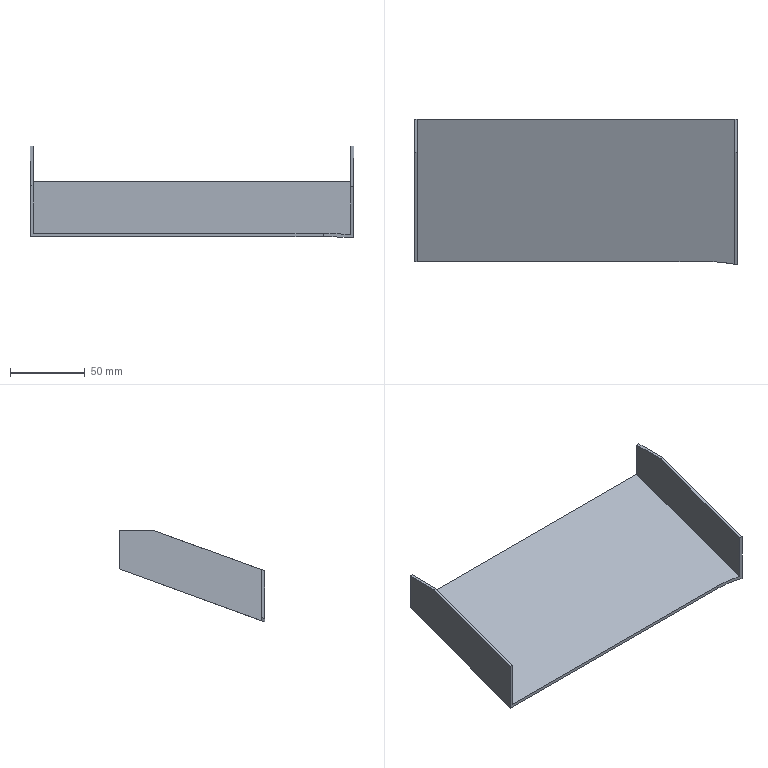Part | NX | features HB 2 | 1 solid | 13 faces | box 216 x 97.247 x 61.333 mm | volume 55606 mm3 | plane 12 | cylinder 1 | commonest cylinder face diameters 190 x1
STEP:
#1=CARTESIAN_POINT('',(865.54,217.702,-213.));
#2=VERTEX_POINT('',#1);
#3=CARTESIAN_POINT('',(865.54,240.,-213.));
#4=VERTEX_POINT('',#3);
#5=CARTESIAN_POINT('',(865.54,20.77,-213.));
#6=DIRECTION('',(0.,1.,0.));
#7=VECTOR('',#6,1000.);
#8=LINE('',#5,#7);
#9=EDGE_CURVE('',#2,#4,#8,.T.);
#10=ORIENTED_EDGE('',*,*,#9,.F.);
#11=CARTESIAN_POINT('',(865.54,142.753,-240.279));
#12=VERTEX_POINT('',#11);
#13=CARTESIAN_POINT('',(865.54,10.51,-288.412));
#14=DIRECTION('',(0.,0.9397,0.342));
#15=VECTOR('',#14,1000.);
#16=LINE('',#13,#15);
#17=EDGE_CURVE('',#12,#2,#16,.T.);
#18=ORIENTED_EDGE('',*,*,#17,.F.);
#19=CARTESIAN_POINT('',(865.54,142.753,-274.333));
#20=VERTEX_POINT('',#19);
#21=CARTESIAN_POINT('',(865.54,142.753,-1420.5));
#22=DIRECTION('',(0.,0.,1.));
#23=VECTOR('',#22,1000.);
#24=LINE('',#21,#23);
#25=EDGE_CURVE('',#20,#12,#24,.T.);
#26=ORIENTED_EDGE('',*,*,#25,.F.);
#27=CARTESIAN_POINT('',(865.54,240.,-238.938));
#28=VERTEX_POINT('',#27);
#29=CARTESIAN_POINT('',(865.54,21.454,-318.482));
#30=DIRECTION('',(0.,-0.9397,-0.342));
#31=VECTOR('',#30,1000.);
#32=LINE('',#29,#31);
#33=EDGE_CURVE('',#28,#20,#32,.T.);
#34=ORIENTED_EDGE('',*,*,#33,.F.);
#35=CARTESIAN_POINT('',(865.54,240.,-316.603));
#36=DIRECTION('',(0.,0.,-1.));
#37=VECTOR('',#36,1000.);
#38=LINE('',#35,#37);
#39=EDGE_CURVE('',#4,#28,#38,.T.);
#40=ORIENTED_EDGE('',*,*,#39,.F.);
#41=EDGE_LOOP('',(#10,#18,#26,#34,#40));
#42=FACE_BOUND('',#41,.T.);
#43=CARTESIAN_POINT('',(865.54,20.77,-316.603));
#44=DIRECTION('',(-1.,0.,0.));
#45=DIRECTION('',(0.,-0.08716,-0.9962));
#46=AXIS2_PLACEMENT_3D('',#43,#44,#45);
#47=PLANE('',#46);
#48=ADVANCED_FACE('',(#42),#47,.F.);
#49=CARTESIAN_POINT('',(649.54,240.,-213.));
#50=VERTEX_POINT('',#49);
#51=CARTESIAN_POINT('',(649.54,217.702,-213.));
#52=VERTEX_POINT('',#51);
#53=CARTESIAN_POINT('',(649.54,20.77,-213.));
#54=DIRECTION('',(0.,-1.,0.));
#55=VECTOR('',#54,1000.);
#56=LINE('',#53,#55);
#57=EDGE_CURVE('',#50,#52,#56,.T.);
#58=ORIENTED_EDGE('',*,*,#57,.F.);
#59=CARTESIAN_POINT('',(649.54,240.,-238.938));
#60=VERTEX_POINT('',#59);
#61=CARTESIAN_POINT('',(649.54,240.,-316.603));
#62=DIRECTION('',(0.,0.,1.));
#63=VECTOR('',#62,1000.);
#64=LINE('',#61,#63);
#65=EDGE_CURVE('',#60,#50,#64,.T.);
#66=ORIENTED_EDGE('',*,*,#65,.F.);
#67=CARTESIAN_POINT('',(649.54,145.,-273.515));
#68=VERTEX_POINT('',#67);
#69=CARTESIAN_POINT('',(649.54,21.454,-318.482));
#70=DIRECTION('',(0.,0.9397,0.342));
#71=VECTOR('',#70,1000.);
#72=LINE('',#69,#71);
#73=EDGE_CURVE('',#68,#60,#72,.T.);
#74=ORIENTED_EDGE('',*,*,#73,.F.);
#75=CARTESIAN_POINT('',(649.54,145.,-239.462));
#76=VERTEX_POINT('',#75);
#77=CARTESIAN_POINT('',(649.54,145.,-316.603));
#78=DIRECTION('',(0.,0.,-1.));
#79=VECTOR('',#78,1000.);
#80=LINE('',#77,#79);
#81=EDGE_CURVE('',#76,#68,#80,.T.);
#82=ORIENTED_EDGE('',*,*,#81,.F.);
#83=CARTESIAN_POINT('',(649.54,10.51,-288.412));
#84=DIRECTION('',(0.,0.9397,0.342));
#85=VECTOR('',#84,1000.);
#86=LINE('',#83,#85);
#87=EDGE_CURVE('',#76,#52,#86,.T.);
#88=ORIENTED_EDGE('',*,*,#87,.T.);
#89=EDGE_LOOP('',(#58,#66,#74,#82,#88));
#90=FACE_BOUND('',#89,.T.);
#91=CARTESIAN_POINT('',(649.54,20.77,-316.603));
#92=DIRECTION('',(1.,0.,0.));
#93=DIRECTION('',(0.,0.08716,0.9962));
#94=AXIS2_PLACEMENT_3D('',#91,#92,#93);
#95=PLANE('',#94);
#96=ADVANCED_FACE('',(#90),#95,.F.);
#97=CARTESIAN_POINT('',(651.54,240.,-236.81));
#98=VERTEX_POINT('',#97);
#99=CARTESIAN_POINT('',(651.54,240.,-213.));
#100=VERTEX_POINT('',#99);
#101=CARTESIAN_POINT('',(651.54,240.,-316.603));
#102=DIRECTION('',(0.,0.,1.));
#103=VECTOR('',#102,1000.);
#104=LINE('',#101,#103);
#105=EDGE_CURVE('',#98,#100,#104,.T.);
#106=ORIENTED_EDGE('',*,*,#105,.T.);
#107=CARTESIAN_POINT('',(651.54,217.702,-213.));
#108=VERTEX_POINT('',#107);
#109=CARTESIAN_POINT('',(651.54,20.77,-213.));
#110=DIRECTION('',(0.,-1.,0.));
#111=VECTOR('',#110,1000.);
#112=LINE('',#109,#111);
#113=EDGE_CURVE('',#100,#108,#112,.T.);
#114=ORIENTED_EDGE('',*,*,#113,.T.);
#115=CARTESIAN_POINT('',(651.54,145.,-239.462));
#116=VERTEX_POINT('',#115);
#117=CARTESIAN_POINT('',(651.54,10.51,-288.412));
#118=DIRECTION('',(0.,0.9397,0.342));
#119=VECTOR('',#118,1000.);
#120=LINE('',#117,#119);
#121=EDGE_CURVE('',#116,#108,#120,.T.);
#122=ORIENTED_EDGE('',*,*,#121,.F.);
#123=CARTESIAN_POINT('',(651.54,145.,-271.387));
#124=VERTEX_POINT('',#123);
#125=CARTESIAN_POINT('',(651.54,145.,-1420.5));
#126=DIRECTION('',(0.,0.,1.));
#127=VECTOR('',#126,1000.);
#128=LINE('',#125,#127);
#129=EDGE_CURVE('',#124,#116,#128,.T.);
#130=ORIENTED_EDGE('',*,*,#129,.F.);
#131=CARTESIAN_POINT('',(651.54,20.77,-316.603));
#132=DIRECTION('',(0.,-0.9397,-0.342));
#133=VECTOR('',#132,1000.);
#134=LINE('',#131,#133);
#135=EDGE_CURVE('',#98,#124,#134,.T.);
#136=ORIENTED_EDGE('',*,*,#135,.F.);
#137=EDGE_LOOP('',(#106,#114,#122,#130,#136));
#138=FACE_BOUND('',#137,.T.);
#139=CARTESIAN_POINT('',(651.54,20.77,-316.603));
#140=DIRECTION('',(1.,0.,0.));
#141=DIRECTION('',(0.,0.08716,0.9962));
#142=AXIS2_PLACEMENT_3D('',#139,#140,#141);
#143=PLANE('',#142);
#144=ADVANCED_FACE('',(#138),#143,.T.);
#145=CARTESIAN_POINT('',(863.54,143.173,-240.126));
#146=VERTEX_POINT('',#145);
#147=CARTESIAN_POINT('',(863.54,217.702,-213.));
#148=VERTEX_POINT('',#147);
#149=CARTESIAN_POINT('',(863.54,10.51,-288.412));
#150=DIRECTION('',(0.,0.9397,0.342));
#151=VECTOR('',#150,1000.);
#152=LINE('',#149,#151);
#153=EDGE_CURVE('',#146,#148,#152,.T.);
#154=ORIENTED_EDGE('',*,*,#153,.T.);
#155=CARTESIAN_POINT('',(863.54,240.,-213.));
#156=VERTEX_POINT('',#155);
#157=CARTESIAN_POINT('',(863.54,20.77,-213.));
#158=DIRECTION('',(0.,1.,0.));
#159=VECTOR('',#158,1000.);
#160=LINE('',#157,#159);
#161=EDGE_CURVE('',#148,#156,#160,.T.);
#162=ORIENTED_EDGE('',*,*,#161,.T.);
#163=CARTESIAN_POINT('',(863.54,240.,-236.81));
#164=VERTEX_POINT('',#163);
#165=CARTESIAN_POINT('',(863.54,240.,-316.603));
#166=DIRECTION('',(0.,0.,-1.));
#167=VECTOR('',#166,1000.);
#168=LINE('',#165,#167);
#169=EDGE_CURVE('',#156,#164,#168,.T.);
#170=ORIENTED_EDGE('',*,*,#169,.T.);
#171=CARTESIAN_POINT('',(863.54,143.173,-272.052));
#172=VERTEX_POINT('',#171);
#173=CARTESIAN_POINT('',(863.54,20.77,-316.603));
#174=DIRECTION('',(0.,0.9397,0.342));
#175=VECTOR('',#174,1000.);
#176=LINE('',#173,#175);
#177=EDGE_CURVE('',#172,#164,#176,.T.);
#178=ORIENTED_EDGE('',*,*,#177,.F.);
#179=CARTESIAN_POINT('',(863.54,143.173,-1420.5));
#180=DIRECTION('',(0.,0.,1.));
#181=VECTOR('',#180,1000.);
#182=LINE('',#179,#181);
#183=EDGE_CURVE('',#172,#146,#182,.T.);
#184=ORIENTED_EDGE('',*,*,#183,.T.);
#185=EDGE_LOOP('',(#154,#162,#170,#178,#184));
#186=FACE_BOUND('',#185,.T.);
#187=CARTESIAN_POINT('',(863.54,20.77,-316.603));
#188=DIRECTION('',(-1.,0.,0.));
#189=DIRECTION('',(0.,0.08716,0.9962));
#190=AXIS2_PLACEMENT_3D('',#187,#188,#189);
#191=PLANE('',#190);
#192=ADVANCED_FACE('',(#186),#191,.T.);
#193=CARTESIAN_POINT('',(651.54,217.702,-213.));
#194=DIRECTION('',(1.,0.,0.));
#195=VECTOR('',#194,1000.);
#196=LINE('',#193,#195);
#197=EDGE_CURVE('',#52,#108,#196,.T.);
#198=ORIENTED_EDGE('',*,*,#197,.F.);
#199=ORIENTED_EDGE('',*,*,#87,.F.);
#200=CARTESIAN_POINT('',(651.54,145.,-239.462));
#201=DIRECTION('',(-1.,0.,0.));
#202=VECTOR('',#201,1000.);
#203=LINE('',#200,#202);
#204=EDGE_CURVE('',#116,#76,#203,.T.);
#205=ORIENTED_EDGE('',*,*,#204,.F.);
#206=ORIENTED_EDGE('',*,*,#121,.T.);
#207=EDGE_LOOP('',(#198,#199,#205,#206));
#208=FACE_BOUND('',#207,.T.);
#209=CARTESIAN_POINT('',(651.54,10.51,-288.412));
#210=DIRECTION('',(0.,0.342,-0.9397));
#211=DIRECTION('',(0.,-0.9397,-0.342));
#212=AXIS2_PLACEMENT_3D('',#209,#210,#211);
#213=PLANE('',#212);
#214=ADVANCED_FACE('',(#208),#213,.F.);
#215=CARTESIAN_POINT('',(973.54,217.702,-213.));
#216=DIRECTION('',(1.,0.,0.));
#217=VECTOR('',#216,1000.);
#218=LINE('',#215,#217);
#219=EDGE_CURVE('',#148,#2,#218,.T.);
#220=ORIENTED_EDGE('',*,*,#219,.F.);
#221=ORIENTED_EDGE('',*,*,#153,.F.);
#222=CARTESIAN_POINT('',(845.,50.,-274.039));
#223=DIRECTION('',(0.,-0.342,0.9397));
#224=DIRECTION('',(0.,0.9397,0.342));
#225=AXIS2_PLACEMENT_3D('',#222,#223,#224);
#226=ELLIPSE('',#225,101.097,95.);
#227=EDGE_CURVE('',#12,#146,#226,.T.);
#228=ORIENTED_EDGE('',*,*,#227,.F.);
#229=ORIENTED_EDGE('',*,*,#17,.T.);
#230=EDGE_LOOP('',(#220,#221,#228,#229));
#231=FACE_BOUND('',#230,.T.);
#232=CARTESIAN_POINT('',(973.54,10.51,-288.412));
#233=DIRECTION('',(0.,0.342,-0.9397));
#234=DIRECTION('',(0.,-0.9397,-0.342));
#235=AXIS2_PLACEMENT_3D('',#232,#233,#234);
#236=PLANE('',#235);
#237=ADVANCED_FACE('',(#231),#236,.F.);
#238=ORIENTED_EDGE('',*,*,#65,.T.);
#239=CARTESIAN_POINT('',(977.,240.,-213.));
#240=DIRECTION('',(1.,0.,0.));
#241=VECTOR('',#240,1000.);
#242=LINE('',#239,#241);
#243=EDGE_CURVE('',#50,#100,#242,.T.);
#244=ORIENTED_EDGE('',*,*,#243,.T.);
#245=ORIENTED_EDGE('',*,*,#105,.F.);
#246=CARTESIAN_POINT('',(868.54,240.,-236.81));
#247=DIRECTION('',(-1.,0.,0.));
#248=VECTOR('',#247,1000.);
#249=LINE('',#246,#248);
#250=EDGE_CURVE('',#164,#98,#249,.T.);
#251=ORIENTED_EDGE('',*,*,#250,.F.);
#252=ORIENTED_EDGE('',*,*,#169,.F.);
#253=CARTESIAN_POINT('',(962.,240.,-213.));
#254=DIRECTION('',(1.,0.,0.));
#255=VECTOR('',#254,1000.);
#256=LINE('',#253,#255);
#257=EDGE_CURVE('',#156,#4,#256,.T.);
#258=ORIENTED_EDGE('',*,*,#257,.T.);
#259=ORIENTED_EDGE('',*,*,#39,.T.);
#260=CARTESIAN_POINT('',(868.54,240.,-238.938));
#261=DIRECTION('',(-1.,0.,0.));
#262=VECTOR('',#261,1000.);
#263=LINE('',#260,#262);
#264=EDGE_CURVE('',#28,#60,#263,.T.);
#265=ORIENTED_EDGE('',*,*,#264,.T.);
#266=EDGE_LOOP('',(#238,#244,#245,#251,#252,#258,#259,#265));
#267=FACE_BOUND('',#266,.T.);
#268=CARTESIAN_POINT('',(962.,240.,60.));
#269=DIRECTION('',(0.,1.,0.));
#270=DIRECTION('',(0.,0.,-1.));
#271=AXIS2_PLACEMENT_3D('',#268,#269,#270);
#272=PLANE('',#271);
#273=ADVANCED_FACE('',(#267),#272,.T.);
#274=ORIENTED_EDGE('',*,*,#135,.T.);
#275=CARTESIAN_POINT('',(845.,145.,-271.387));
#276=VERTEX_POINT('',#275);
#277=CARTESIAN_POINT('',(868.54,145.,-271.387));
#278=DIRECTION('',(1.,0.,0.));
#279=VECTOR('',#278,1000.);
#280=LINE('',#277,#279);
#281=EDGE_CURVE('',#124,#276,#280,.T.);
#282=ORIENTED_EDGE('',*,*,#281,.T.);
#283=CARTESIAN_POINT('',(845.,50.,-305.964));
#284=DIRECTION('',(0.,-0.342,0.9397));
#285=DIRECTION('',(0.,0.9397,0.342));
#286=AXIS2_PLACEMENT_3D('',#283,#284,#285);
#287=ELLIPSE('',#286,101.097,95.);
#288=EDGE_CURVE('',#172,#276,#287,.T.);
#289=ORIENTED_EDGE('',*,*,#288,.F.);
#290=ORIENTED_EDGE('',*,*,#177,.T.);
#291=ORIENTED_EDGE('',*,*,#250,.T.);
#292=EDGE_LOOP('',(#274,#282,#289,#290,#291));
#293=FACE_BOUND('',#292,.T.);
#294=CARTESIAN_POINT('',(868.54,20.77,-316.603));
#295=DIRECTION('',(0.,-0.342,0.9397));
#296=DIRECTION('',(-1.,0.,0.));
#297=AXIS2_PLACEMENT_3D('',#294,#295,#296);
#298=PLANE('',#297);
#299=ADVANCED_FACE('',(#293),#298,.T.);
#300=CARTESIAN_POINT('',(845.,145.,-273.515));
#301=VERTEX_POINT('',#300);
#302=CARTESIAN_POINT('',(868.54,145.,-273.515));
#303=DIRECTION('',(-1.,0.,0.));
#304=VECTOR('',#303,1000.);
#305=LINE('',#302,#304);
#306=EDGE_CURVE('',#301,#68,#305,.T.);
#307=ORIENTED_EDGE('',*,*,#306,.T.);
#308=ORIENTED_EDGE('',*,*,#73,.T.);
#309=ORIENTED_EDGE('',*,*,#264,.F.);
#310=ORIENTED_EDGE('',*,*,#33,.T.);
#311=CARTESIAN_POINT('',(845.,50.,-308.092));
#312=DIRECTION('',(0.,-0.342,0.9397));
#313=DIRECTION('',(0.,0.9397,0.342));
#314=AXIS2_PLACEMENT_3D('',#311,#312,#313);
#315=ELLIPSE('',#314,101.097,95.);
#316=EDGE_CURVE('',#20,#301,#315,.T.);
#317=ORIENTED_EDGE('',*,*,#316,.T.);
#318=EDGE_LOOP('',(#307,#308,#309,#310,#317));
#319=FACE_BOUND('',#318,.T.);
#320=CARTESIAN_POINT('',(868.54,21.454,-318.482));
#321=DIRECTION('',(0.,-0.342,0.9397));
#322=DIRECTION('',(-1.,0.,0.));
#323=AXIS2_PLACEMENT_3D('',#320,#321,#322);
#324=PLANE('',#323);
#325=ADVANCED_FACE('',(#319),#324,.F.);
#326=ORIENTED_EDGE('',*,*,#281,.F.);
#327=ORIENTED_EDGE('',*,*,#129,.T.);
#328=ORIENTED_EDGE('',*,*,#204,.T.);
#329=ORIENTED_EDGE('',*,*,#81,.T.);
#330=ORIENTED_EDGE('',*,*,#306,.F.);
#331=CARTESIAN_POINT('',(845.,145.,-1420.5));
#332=DIRECTION('',(0.,0.,1.));
#333=VECTOR('',#332,1000.);
#334=LINE('',#331,#333);
#335=EDGE_CURVE('',#301,#276,#334,.T.);
#336=ORIENTED_EDGE('',*,*,#335,.T.);
#337=EDGE_LOOP('',(#326,#327,#328,#329,#330,#336));
#338=FACE_BOUND('',#337,.T.);
#339=CARTESIAN_POINT('',(645.,145.,-1420.5));
#340=DIRECTION('',(0.,-1.,0.));
#341=DIRECTION('',(0.,0.,1.));
#342=AXIS2_PLACEMENT_3D('',#339,#340,#341);
#343=PLANE('',#342);
#344=ADVANCED_FACE('',(#338),#343,.T.);
#345=ORIENTED_EDGE('',*,*,#288,.T.);
#346=ORIENTED_EDGE('',*,*,#335,.F.);
#347=ORIENTED_EDGE('',*,*,#316,.F.);
#348=ORIENTED_EDGE('',*,*,#25,.T.);
#349=ORIENTED_EDGE('',*,*,#227,.T.);
#350=ORIENTED_EDGE('',*,*,#183,.F.);
#351=EDGE_LOOP('',(#345,#346,#347,#348,#349,#350));
#352=FACE_BOUND('',#351,.T.);
#353=CARTESIAN_POINT('',(845.,50.,-1420.5));
#354=DIRECTION('',(0.,0.,1.));
#355=DIRECTION('',(-1.,0.,0.));
#356=AXIS2_PLACEMENT_3D('',#353,#354,#355);
#357=CYLINDRICAL_SURFACE('',#356,95.);
#358=ADVANCED_FACE('',(#352),#357,.F.);
#359=ORIENTED_EDGE('',*,*,#161,.F.);
#360=ORIENTED_EDGE('',*,*,#219,.T.);
#361=ORIENTED_EDGE('',*,*,#9,.T.);
#362=ORIENTED_EDGE('',*,*,#257,.F.);
#363=EDGE_LOOP('',(#359,#360,#361,#362));
#364=FACE_BOUND('',#363,.T.);
#365=CARTESIAN_POINT('',(1945.,0.,-213.));
#366=DIRECTION('',(0.,0.,1.));
#367=DIRECTION('',(-1.,0.,0.));
#368=AXIS2_PLACEMENT_3D('',#365,#366,#367);
#369=PLANE('',#368);
#370=ADVANCED_FACE('',(#364),#369,.T.);
#371=ORIENTED_EDGE('',*,*,#57,.T.);
#372=ORIENTED_EDGE('',*,*,#197,.T.);
#373=ORIENTED_EDGE('',*,*,#113,.F.);
#374=ORIENTED_EDGE('',*,*,#243,.F.);
#375=EDGE_LOOP('',(#371,#372,#373,#374));
#376=FACE_BOUND('',#375,.T.);
#377=CARTESIAN_POINT('',(1960.,0.,-213.));
#378=DIRECTION('',(0.,0.,1.));
#379=DIRECTION('',(-1.,0.,0.));
#380=AXIS2_PLACEMENT_3D('',#377,#378,#379);
#381=PLANE('',#380);
#382=ADVANCED_FACE('',(#376),#381,.T.);
#383=CLOSED_SHELL('',(#48,#96,#144,#192,#214,#237,#273,#299,#325,#344,#358,#370,#382));
#384=MANIFOLD_SOLID_BREP('',#383);
#385=(LENGTH_UNIT()NAMED_UNIT(*)SI_UNIT(.MILLI.,.METRE.));
#386=UNCERTAINTY_MEASURE_WITH_UNIT(LENGTH_MEASURE(0.00001),#385,'','');
#387=(NAMED_UNIT(*)PLANE_ANGLE_UNIT()SI_UNIT($,.RADIAN.));
#388=(NAMED_UNIT(*)SI_UNIT($,.STERADIAN.)SOLID_ANGLE_UNIT());
#389=(GEOMETRIC_REPRESENTATION_CONTEXT(3)GLOBAL_UNCERTAINTY_ASSIGNED_CONTEXT((#386))GLOBAL_UNIT_ASSIGNED_CONTEXT((#385,#387,#388))REPRESENTATION_CONTEXT('',''));
#390=ADVANCED_BREP_SHAPE_REPRESENTATION('',(#384),#389);